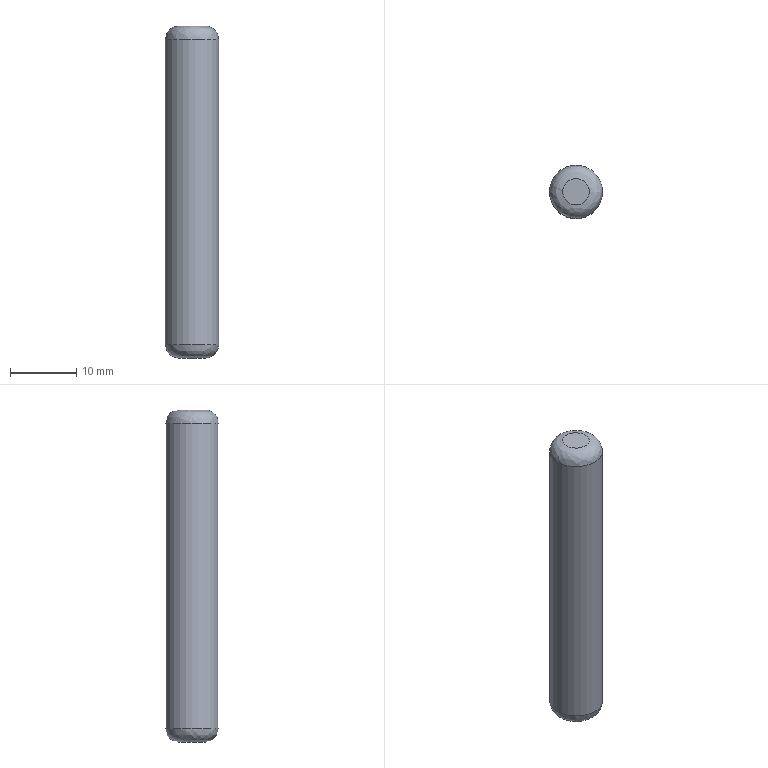Part | STEP file | 1 solid | 5 faces | box 8 x 8 x 50 mm | volume 2474 mm3 | plane 2 | spline 2 | cylinder 1 | commonest cylinder face diameters 8 x1
STEP:
#1=CARTESIAN_POINT('',(0.,0.,0.));
#2=DIRECTION('',(0.,0.,1.));
#3=DIRECTION('',(1.,0.,0.));
#4=AXIS2_PLACEMENT_3D('',#1,#2,#3);
#5=CARTESIAN_POINT('',(1296.247,499.955,58.619));
#6=VERTEX_POINT('',#5);
#7=CARTESIAN_POINT('',(1292.247,499.955,58.619));
#8=DIRECTION('',(0.,0.,-1.));
#9=DIRECTION('',(1.,0.,0.));
#10=AXIS2_PLACEMENT_3D('',#7,#8,#9);
#11=CIRCLE('',#10,4.);
#12=CARTESIAN_POINT('',(1292.247,499.955,10.619));
#13=DIRECTION('',(0.,0.,1.));
#14=DIRECTION('',(1.,0.,0.));
#15=AXIS2_PLACEMENT_3D('',#12,#13,#14);
#16=CYLINDRICAL_SURFACE('',#15,4.);
#17=CARTESIAN_POINT('',(6.283,48.));
#18=DIRECTION('',(-1.,0.));
#19=VECTOR('',#18,1.);
#20=LINE('',#17,#19);
#21=(GEOMETRIC_REPRESENTATION_CONTEXT(2)PARAMETRIC_REPRESENTATION_CONTEXT()REPRESENTATION_CONTEXT('',''));
#22=DEFINITIONAL_REPRESENTATION('',(#20),#21);
#23=PCURVE('',#16,#22);
#24=CARTESIAN_POINT('',(1288.247,499.955,58.619));
#25=CARTESIAN_POINT('',(1288.247,507.955,58.619));
#26=CARTESIAN_POINT('',(1296.247,507.955,58.619));
#27=CARTESIAN_POINT('',(1296.247,499.955,58.619));
#28=CARTESIAN_POINT('',(1296.247,491.955,58.619));
#29=CARTESIAN_POINT('',(1288.247,491.955,58.619));
#30=CARTESIAN_POINT('',(1288.247,499.955,58.619));
#31=CARTESIAN_POINT('',(1288.247,499.955,59.791));
#32=CARTESIAN_POINT('',(1288.247,507.955,59.791));
#33=CARTESIAN_POINT('',(1296.247,507.955,59.791));
#34=CARTESIAN_POINT('',(1296.247,499.955,59.791));
#35=CARTESIAN_POINT('',(1296.247,491.955,59.791));
#36=CARTESIAN_POINT('',(1288.247,491.955,59.791));
#37=CARTESIAN_POINT('',(1288.247,499.955,59.791));
#38=CARTESIAN_POINT('',(1289.076,499.955,60.619));
#39=CARTESIAN_POINT('',(1289.076,506.299,60.619));
#40=CARTESIAN_POINT('',(1295.419,506.299,60.619));
#41=CARTESIAN_POINT('',(1295.419,499.955,60.619));
#42=CARTESIAN_POINT('',(1295.419,493.612,60.619));
#43=CARTESIAN_POINT('',(1289.076,493.612,60.619));
#44=CARTESIAN_POINT('',(1289.076,499.955,60.619));
#45=CARTESIAN_POINT('',(1290.247,499.955,60.619));
#46=CARTESIAN_POINT('',(1290.247,503.955,60.619));
#47=CARTESIAN_POINT('',(1294.247,503.955,60.619));
#48=CARTESIAN_POINT('',(1294.247,499.955,60.619));
#49=CARTESIAN_POINT('',(1294.247,495.955,60.619));
#50=CARTESIAN_POINT('',(1290.247,495.955,60.619));
#51=CARTESIAN_POINT('',(1290.247,499.955,60.619));
#52=(BOUNDED_SURFACE()B_SPLINE_SURFACE(3,3,((#24,#25,#26,#27,#28,#29,#30),(#31,#32,#33,#34,#35,#36,#37),(#38,#39,#40,#41,#42,#43,#44),(#45,#46,#47,#48,#49,#50,#51)),.UNSPECIFIED.,.F.,.T.,.F.)B_SPLINE_SURFACE_WITH_KNOTS((4,4),(1,3,3,3,1),(0.,1.),(-0.5,0.,0.5,1.,1.5),.UNSPECIFIED.)GEOMETRIC_REPRESENTATION_ITEM()RATIONAL_B_SPLINE_SURFACE(((1.,0.3333,0.3333,1.,0.3333,0.3333,1.),(0.8047,0.2682,0.2682,0.8047,0.2682,0.2682,0.8047),(0.8047,0.2682,0.2682,0.8047,0.2682,0.2682,0.8047),(1.,0.3333,0.3333,1.,0.3333,0.3333,1.)))REPRESENTATION_ITEM('')SURFACE());
#53=CARTESIAN_POINT('',(0.,0.5));
#54=CARTESIAN_POINT('',(0.,0.5235));
#55=CARTESIAN_POINT('',(0.,0.5649));
#56=CARTESIAN_POINT('',(0.,0.6146));
#57=CARTESIAN_POINT('',(0.,0.6575));
#58=CARTESIAN_POINT('',(0.,0.696));
#59=CARTESIAN_POINT('',(0.,0.7322));
#60=CARTESIAN_POINT('',(0.,0.7678));
#61=CARTESIAN_POINT('',(0.,0.804));
#62=CARTESIAN_POINT('',(0.,0.8425));
#63=CARTESIAN_POINT('',(0.,0.8856));
#64=CARTESIAN_POINT('',(0.,0.9343));
#65=CARTESIAN_POINT('',(0.,1.));
#66=CARTESIAN_POINT('',(0.,1.066));
#67=CARTESIAN_POINT('',(0.,1.114));
#68=CARTESIAN_POINT('',(0.,1.158));
#69=CARTESIAN_POINT('',(0.,1.196));
#70=CARTESIAN_POINT('',(0.,1.232));
#71=CARTESIAN_POINT('',(0.,1.268));
#72=CARTESIAN_POINT('',(0.,1.304));
#73=CARTESIAN_POINT('',(0.,1.343));
#74=CARTESIAN_POINT('',(0.,1.385));
#75=CARTESIAN_POINT('',(0.,1.435));
#76=CARTESIAN_POINT('',(0.,1.476));
#77=CARTESIAN_POINT('',(0.,1.5));
#78=B_SPLINE_CURVE_WITH_KNOTS('',3,(#53,#54,#55,#56,#57,#58,#59,#60,#61,#62,#63,#64,#65,#66,#67,#68,#69,#70,#71,#72,#73,#74,#75,#76,#77),.UNSPECIFIED.,.F.,.F.,(4,1,1,1,1,1,1,1,1,1,1,1,1,1,1,1,1,1,1,1,1,1,4),(0.,0.2856,0.5712,0.8568,1.142,1.428,1.714,1.999,2.285,2.57,2.856,3.142,3.427,3.713,3.998,4.284,4.57,4.855,5.141,5.426,5.712,5.998,6.283),.QUASI_UNIFORM_KNOTS.);
#79=(GEOMETRIC_REPRESENTATION_CONTEXT(2)PARAMETRIC_REPRESENTATION_CONTEXT()REPRESENTATION_CONTEXT('',''));
#80=DEFINITIONAL_REPRESENTATION('',(#78),#79);
#81=PCURVE('',#52,#80);
#82=SURFACE_CURVE('',#11,(#23,#81),.PCURVE_S1.);
#83=EDGE_CURVE('',#6,#6,#82,.T.);
#84=ORIENTED_EDGE('',*,*,#83,.T.);
#85=CARTESIAN_POINT('',(1296.247,499.955,12.619));
#86=VERTEX_POINT('',#85);
#87=CARTESIAN_POINT('',(1296.247,499.955,12.619));
#88=CARTESIAN_POINT('',(1296.247,499.955,58.619));
#89=B_SPLINE_CURVE_WITH_KNOTS('',1,(#87,#88),.UNSPECIFIED.,.F.,.F.,(2,2),(2.,48.),.PIECEWISE_BEZIER_KNOTS.);
#90=CARTESIAN_POINT('',(0.,0.));
#91=DIRECTION('',(0.,1.));
#92=VECTOR('',#91,1.);
#93=LINE('',#90,#92);
#94=(GEOMETRIC_REPRESENTATION_CONTEXT(2)PARAMETRIC_REPRESENTATION_CONTEXT()REPRESENTATION_CONTEXT('',''));
#95=DEFINITIONAL_REPRESENTATION('',(#93),#94);
#96=PCURVE('',#16,#95);
#97=CARTESIAN_POINT('',(6.283,0.));
#98=DIRECTION('',(0.,1.));
#99=VECTOR('',#98,1.);
#100=LINE('',#97,#99);
#101=(GEOMETRIC_REPRESENTATION_CONTEXT(2)PARAMETRIC_REPRESENTATION_CONTEXT()REPRESENTATION_CONTEXT('',''));
#102=DEFINITIONAL_REPRESENTATION('',(#100),#101);
#103=PCURVE('',#16,#102);
#104=SEAM_CURVE('',#89,(#96,#103),.PCURVE_S1.);
#105=EDGE_CURVE('',#86,#6,#104,.T.);
#106=ORIENTED_EDGE('',*,*,#105,.F.);
#107=CARTESIAN_POINT('',(1292.247,499.955,12.619));
#108=DIRECTION('',(0.,0.,1.));
#109=DIRECTION('',(1.,0.,0.));
#110=AXIS2_PLACEMENT_3D('',#107,#108,#109);
#111=CIRCLE('',#110,4.);
#112=CARTESIAN_POINT('',(0.,2.));
#113=DIRECTION('',(1.,0.));
#114=VECTOR('',#113,1.);
#115=LINE('',#112,#114);
#116=(GEOMETRIC_REPRESENTATION_CONTEXT(2)PARAMETRIC_REPRESENTATION_CONTEXT()REPRESENTATION_CONTEXT('',''));
#117=DEFINITIONAL_REPRESENTATION('',(#115),#116);
#118=PCURVE('',#16,#117);
#119=CARTESIAN_POINT('',(1290.247,499.955,10.619));
#120=CARTESIAN_POINT('',(1290.247,503.955,10.619));
#121=CARTESIAN_POINT('',(1294.247,503.955,10.619));
#122=CARTESIAN_POINT('',(1294.247,499.955,10.619));
#123=CARTESIAN_POINT('',(1294.247,495.955,10.619));
#124=CARTESIAN_POINT('',(1290.247,495.955,10.619));
#125=CARTESIAN_POINT('',(1290.247,499.955,10.619));
#126=CARTESIAN_POINT('',(1289.076,499.955,10.619));
#127=CARTESIAN_POINT('',(1289.076,506.299,10.619));
#128=CARTESIAN_POINT('',(1295.419,506.299,10.619));
#129=CARTESIAN_POINT('',(1295.419,499.955,10.619));
#130=CARTESIAN_POINT('',(1295.419,493.612,10.619));
#131=CARTESIAN_POINT('',(1289.076,493.612,10.619));
#132=CARTESIAN_POINT('',(1289.076,499.955,10.619));
#133=CARTESIAN_POINT('',(1288.247,499.955,11.447));
#134=CARTESIAN_POINT('',(1288.247,507.955,11.447));
#135=CARTESIAN_POINT('',(1296.247,507.955,11.447));
#136=CARTESIAN_POINT('',(1296.247,499.955,11.447));
#137=CARTESIAN_POINT('',(1296.247,491.955,11.447));
#138=CARTESIAN_POINT('',(1288.247,491.955,11.447));
#139=CARTESIAN_POINT('',(1288.247,499.955,11.447));
#140=CARTESIAN_POINT('',(1288.247,499.955,12.619));
#141=CARTESIAN_POINT('',(1288.247,507.955,12.619));
#142=CARTESIAN_POINT('',(1296.247,507.955,12.619));
#143=CARTESIAN_POINT('',(1296.247,499.955,12.619));
#144=CARTESIAN_POINT('',(1296.247,491.955,12.619));
#145=CARTESIAN_POINT('',(1288.247,491.955,12.619));
#146=CARTESIAN_POINT('',(1288.247,499.955,12.619));
#147=(BOUNDED_SURFACE()B_SPLINE_SURFACE(3,3,((#119,#120,#121,#122,#123,#124,#125),(#126,#127,#128,#129,#130,#131,#132),(#133,#134,#135,#136,#137,#138,#139),(#140,#141,#142,#143,#144,#145,#146)),.UNSPECIFIED.,.F.,.T.,.F.)B_SPLINE_SURFACE_WITH_KNOTS((4,4),(1,3,3,3,1),(0.,1.),(-0.5,0.,0.5,1.,1.5),.UNSPECIFIED.)GEOMETRIC_REPRESENTATION_ITEM()RATIONAL_B_SPLINE_SURFACE(((1.,0.3333,0.3333,1.,0.3333,0.3333,1.),(0.8047,0.2682,0.2682,0.8047,0.2682,0.2682,0.8047),(0.8047,0.2682,0.2682,0.8047,0.2682,0.2682,0.8047),(1.,0.3333,0.3333,1.,0.3333,0.3333,1.)))REPRESENTATION_ITEM('')SURFACE());
#148=CARTESIAN_POINT('',(1.,1.5));
#149=CARTESIAN_POINT('',(1.,1.476));
#150=CARTESIAN_POINT('',(1.,1.435));
#151=CARTESIAN_POINT('',(1.,1.385));
#152=CARTESIAN_POINT('',(1.,1.343));
#153=CARTESIAN_POINT('',(1.,1.304));
#154=CARTESIAN_POINT('',(1.,1.268));
#155=CARTESIAN_POINT('',(1.,1.232));
#156=CARTESIAN_POINT('',(1.,1.196));
#157=CARTESIAN_POINT('',(1.,1.158));
#158=CARTESIAN_POINT('',(1.,1.114));
#159=CARTESIAN_POINT('',(1.,1.066));
#160=CARTESIAN_POINT('',(1.,1.));
#161=CARTESIAN_POINT('',(1.,0.9343));
#162=CARTESIAN_POINT('',(1.,0.8856));
#163=CARTESIAN_POINT('',(1.,0.8425));
#164=CARTESIAN_POINT('',(1.,0.804));
#165=CARTESIAN_POINT('',(1.,0.7678));
#166=CARTESIAN_POINT('',(1.,0.7322));
#167=CARTESIAN_POINT('',(1.,0.696));
#168=CARTESIAN_POINT('',(1.,0.6575));
#169=CARTESIAN_POINT('',(1.,0.6146));
#170=CARTESIAN_POINT('',(1.,0.5649));
#171=CARTESIAN_POINT('',(1.,0.5235));
#172=CARTESIAN_POINT('',(1.,0.5));
#173=B_SPLINE_CURVE_WITH_KNOTS('',3,(#148,#149,#150,#151,#152,#153,#154,#155,#156,#157,#158,#159,#160,#161,#162,#163,#164,#165,#166,#167,#168,#169,#170,#171,#172),.UNSPECIFIED.,.F.,.F.,(4,1,1,1,1,1,1,1,1,1,1,1,1,1,1,1,1,1,1,1,1,1,4),(0.,0.2856,0.5712,0.8568,1.142,1.428,1.714,1.999,2.285,2.57,2.856,3.142,3.427,3.713,3.998,4.284,4.57,4.855,5.141,5.426,5.712,5.998,6.283),.QUASI_UNIFORM_KNOTS.);
#174=(GEOMETRIC_REPRESENTATION_CONTEXT(2)PARAMETRIC_REPRESENTATION_CONTEXT()REPRESENTATION_CONTEXT('',''));
#175=DEFINITIONAL_REPRESENTATION('',(#173),#174);
#176=PCURVE('',#147,#175);
#177=SURFACE_CURVE('',#111,(#118,#176),.PCURVE_S1.);
#178=EDGE_CURVE('',#86,#86,#177,.T.);
#179=ORIENTED_EDGE('',*,*,#178,.T.);
#180=ORIENTED_EDGE('',*,*,#105,.T.);
#181=EDGE_LOOP('',(#84,#106,#179,#180));
#182=FACE_BOUND('',#181,.T.);
#183=ADVANCED_FACE('',(#182),#16,.T.);
#184=CARTESIAN_POINT('',(1294.247,499.955,10.619));
#185=VERTEX_POINT('',#184);
#186=CARTESIAN_POINT('',(1292.247,499.955,10.619));
#187=DIRECTION('',(0.,0.,-1.));
#188=DIRECTION('',(1.,0.,0.));
#189=AXIS2_PLACEMENT_3D('',#186,#187,#188);
#190=CIRCLE('',#189,2.);
#191=CARTESIAN_POINT('',(1292.247,499.955,10.619));
#192=DIRECTION('',(0.,0.,-1.));
#193=DIRECTION('',(-1.,0.,0.));
#194=AXIS2_PLACEMENT_3D('',#191,#192,#193);
#195=PLANE('',#194);
#196=CARTESIAN_POINT('',(0.,0.));
#197=DIRECTION('',(-1.,0.));
#198=AXIS2_PLACEMENT_2D('',#196,#197);
#199=CIRCLE('',#198,2.);
#200=(GEOMETRIC_REPRESENTATION_CONTEXT(2)PARAMETRIC_REPRESENTATION_CONTEXT()REPRESENTATION_CONTEXT('',''));
#201=DEFINITIONAL_REPRESENTATION('',(#199),#200);
#202=PCURVE('',#195,#201);
#203=CARTESIAN_POINT('',(0.,0.5));
#204=CARTESIAN_POINT('',(0.,0.5235));
#205=CARTESIAN_POINT('',(0.,0.5649));
#206=CARTESIAN_POINT('',(0.,0.6146));
#207=CARTESIAN_POINT('',(0.,0.6575));
#208=CARTESIAN_POINT('',(0.,0.696));
#209=CARTESIAN_POINT('',(0.,0.7322));
#210=CARTESIAN_POINT('',(0.,0.7678));
#211=CARTESIAN_POINT('',(0.,0.804));
#212=CARTESIAN_POINT('',(0.,0.8425));
#213=CARTESIAN_POINT('',(0.,0.8856));
#214=CARTESIAN_POINT('',(0.,0.9343));
#215=CARTESIAN_POINT('',(0.,1.));
#216=CARTESIAN_POINT('',(0.,1.066));
#217=CARTESIAN_POINT('',(0.,1.114));
#218=CARTESIAN_POINT('',(0.,1.158));
#219=CARTESIAN_POINT('',(0.,1.196));
#220=CARTESIAN_POINT('',(0.,1.232));
#221=CARTESIAN_POINT('',(0.,1.268));
#222=CARTESIAN_POINT('',(0.,1.304));
#223=CARTESIAN_POINT('',(0.,1.343));
#224=CARTESIAN_POINT('',(0.,1.385));
#225=CARTESIAN_POINT('',(0.,1.435));
#226=CARTESIAN_POINT('',(0.,1.476));
#227=CARTESIAN_POINT('',(0.,1.5));
#228=B_SPLINE_CURVE_WITH_KNOTS('',3,(#203,#204,#205,#206,#207,#208,#209,#210,#211,#212,#213,#214,#215,#216,#217,#218,#219,#220,#221,#222,#223,#224,#225,#226,#227),.UNSPECIFIED.,.F.,.F.,(4,1,1,1,1,1,1,1,1,1,1,1,1,1,1,1,1,1,1,1,1,1,4),(0.,0.2856,0.5712,0.8568,1.142,1.428,1.714,1.999,2.285,2.57,2.856,3.142,3.427,3.713,3.998,4.284,4.57,4.855,5.141,5.426,5.712,5.998,6.283),.QUASI_UNIFORM_KNOTS.);
#229=(GEOMETRIC_REPRESENTATION_CONTEXT(2)PARAMETRIC_REPRESENTATION_CONTEXT()REPRESENTATION_CONTEXT('',''));
#230=DEFINITIONAL_REPRESENTATION('',(#228),#229);
#231=PCURVE('',#147,#230);
#232=SURFACE_CURVE('',#190,(#202,#231),.PCURVE_S1.);
#233=EDGE_CURVE('',#185,#185,#232,.T.);
#234=ORIENTED_EDGE('',*,*,#233,.T.);
#235=EDGE_LOOP('',(#234));
#236=FACE_BOUND('',#235,.T.);
#237=ADVANCED_FACE('',(#236),#195,.T.);
#238=CARTESIAN_POINT('',(1294.247,499.955,60.619));
#239=VERTEX_POINT('',#238);
#240=CARTESIAN_POINT('',(1292.247,499.955,60.619));
#241=DIRECTION('',(0.,0.,1.));
#242=DIRECTION('',(1.,0.,0.));
#243=AXIS2_PLACEMENT_3D('',#240,#241,#242);
#244=CIRCLE('',#243,2.);
#245=CARTESIAN_POINT('',(1292.247,499.955,60.619));
#246=DIRECTION('',(0.,0.,-1.));
#247=DIRECTION('',(-1.,0.,0.));
#248=AXIS2_PLACEMENT_3D('',#245,#246,#247);
#249=PLANE('',#248);
#250=CARTESIAN_POINT('',(-2.,0.));
#251=CARTESIAN_POINT('',(-2.,3.464));
#252=CARTESIAN_POINT('',(1.,1.732));
#253=CARTESIAN_POINT('',(4.,0.));
#254=CARTESIAN_POINT('',(1.,-1.732));
#255=CARTESIAN_POINT('',(-2.,-3.464));
#256=CARTESIAN_POINT('',(-2.,0.));
#257=(BOUNDED_CURVE()B_SPLINE_CURVE(2,(#250,#251,#252,#253,#254,#255,#256),.UNSPECIFIED.,.T.,.F.)B_SPLINE_CURVE_WITH_KNOTS((1,2,2,2,2,1),(-2.094,0.,2.094,4.189,6.283,8.378),.UNSPECIFIED.)CURVE()GEOMETRIC_REPRESENTATION_ITEM()RATIONAL_B_SPLINE_CURVE((1.,0.5,1.,0.5,1.,0.5,1.))REPRESENTATION_ITEM(''));
#258=(GEOMETRIC_REPRESENTATION_CONTEXT(2)PARAMETRIC_REPRESENTATION_CONTEXT()REPRESENTATION_CONTEXT('',''));
#259=DEFINITIONAL_REPRESENTATION('',(#257),#258);
#260=PCURVE('',#249,#259);
#261=CARTESIAN_POINT('',(1.,1.5));
#262=CARTESIAN_POINT('',(1.,1.476));
#263=CARTESIAN_POINT('',(1.,1.435));
#264=CARTESIAN_POINT('',(1.,1.385));
#265=CARTESIAN_POINT('',(1.,1.343));
#266=CARTESIAN_POINT('',(1.,1.304));
#267=CARTESIAN_POINT('',(1.,1.268));
#268=CARTESIAN_POINT('',(1.,1.232));
#269=CARTESIAN_POINT('',(1.,1.196));
#270=CARTESIAN_POINT('',(1.,1.158));
#271=CARTESIAN_POINT('',(1.,1.114));
#272=CARTESIAN_POINT('',(1.,1.066));
#273=CARTESIAN_POINT('',(1.,1.));
#274=CARTESIAN_POINT('',(1.,0.9343));
#275=CARTESIAN_POINT('',(1.,0.8856));
#276=CARTESIAN_POINT('',(1.,0.8425));
#277=CARTESIAN_POINT('',(1.,0.804));
#278=CARTESIAN_POINT('',(1.,0.7678));
#279=CARTESIAN_POINT('',(1.,0.7322));
#280=CARTESIAN_POINT('',(1.,0.696));
#281=CARTESIAN_POINT('',(1.,0.6575));
#282=CARTESIAN_POINT('',(1.,0.6146));
#283=CARTESIAN_POINT('',(1.,0.5649));
#284=CARTESIAN_POINT('',(1.,0.5235));
#285=CARTESIAN_POINT('',(1.,0.5));
#286=B_SPLINE_CURVE_WITH_KNOTS('',3,(#261,#262,#263,#264,#265,#266,#267,#268,#269,#270,#271,#272,#273,#274,#275,#276,#277,#278,#279,#280,#281,#282,#283,#284,#285),.UNSPECIFIED.,.F.,.F.,(4,1,1,1,1,1,1,1,1,1,1,1,1,1,1,1,1,1,1,1,1,1,4),(0.,0.2856,0.5712,0.8568,1.142,1.428,1.714,1.999,2.285,2.57,2.856,3.142,3.427,3.713,3.998,4.284,4.57,4.855,5.141,5.426,5.712,5.998,6.283),.QUASI_UNIFORM_KNOTS.);
#287=(GEOMETRIC_REPRESENTATION_CONTEXT(2)PARAMETRIC_REPRESENTATION_CONTEXT()REPRESENTATION_CONTEXT('',''));
#288=DEFINITIONAL_REPRESENTATION('',(#286),#287);
#289=PCURVE('',#52,#288);
#290=SURFACE_CURVE('',#244,(#260,#289),.PCURVE_S1.);
#291=EDGE_CURVE('',#239,#239,#290,.T.);
#292=ORIENTED_EDGE('',*,*,#291,.T.);
#293=EDGE_LOOP('',(#292));
#294=FACE_BOUND('',#293,.T.);
#295=ADVANCED_FACE('',(#294),#249,.F.);
#296=ORIENTED_EDGE('',*,*,#291,.F.);
#297=CARTESIAN_POINT('',(1296.247,499.955,58.619));
#298=CARTESIAN_POINT('',(1296.247,499.955,59.791));
#299=CARTESIAN_POINT('',(1295.419,499.955,60.619));
#300=CARTESIAN_POINT('',(1294.247,499.955,60.619));
#301=(BOUNDED_CURVE()B_SPLINE_CURVE(3,(#297,#298,#299,#300),.UNSPECIFIED.,.F.,.F.)B_SPLINE_CURVE_WITH_KNOTS((4,4),(0.,1.),.PIECEWISE_BEZIER_KNOTS.)CURVE()GEOMETRIC_REPRESENTATION_ITEM()RATIONAL_B_SPLINE_CURVE((1.,0.8047,0.8047,1.))REPRESENTATION_ITEM(''));
#302=CARTESIAN_POINT('',(0.,1.5));
#303=DIRECTION('',(1.,0.));
#304=VECTOR('',#303,1.);
#305=LINE('',#302,#304);
#306=(GEOMETRIC_REPRESENTATION_CONTEXT(2)PARAMETRIC_REPRESENTATION_CONTEXT()REPRESENTATION_CONTEXT('',''));
#307=DEFINITIONAL_REPRESENTATION('',(#305),#306);
#308=PCURVE('',#52,#307);
#309=CARTESIAN_POINT('',(0.,0.5));
#310=DIRECTION('',(1.,0.));
#311=VECTOR('',#310,1.);
#312=LINE('',#309,#311);
#313=(GEOMETRIC_REPRESENTATION_CONTEXT(2)PARAMETRIC_REPRESENTATION_CONTEXT()REPRESENTATION_CONTEXT('',''));
#314=DEFINITIONAL_REPRESENTATION('',(#312),#313);
#315=PCURVE('',#52,#314);
#316=SEAM_CURVE('',#301,(#308,#315),.PCURVE_S1.);
#317=EDGE_CURVE('',#6,#239,#316,.T.);
#318=ORIENTED_EDGE('',*,*,#317,.F.);
#319=ORIENTED_EDGE('',*,*,#83,.F.);
#320=ORIENTED_EDGE('',*,*,#317,.T.);
#321=EDGE_LOOP('',(#296,#318,#319,#320));
#322=FACE_BOUND('',#321,.T.);
#323=ADVANCED_FACE('',(#322),#52,.T.);
#324=ORIENTED_EDGE('',*,*,#178,.F.);
#325=CARTESIAN_POINT('',(1294.247,499.955,10.619));
#326=CARTESIAN_POINT('',(1295.419,499.955,10.619));
#327=CARTESIAN_POINT('',(1296.247,499.955,11.447));
#328=CARTESIAN_POINT('',(1296.247,499.955,12.619));
#329=(BOUNDED_CURVE()B_SPLINE_CURVE(3,(#325,#326,#327,#328),.UNSPECIFIED.,.F.,.F.)B_SPLINE_CURVE_WITH_KNOTS((4,4),(0.,1.),.PIECEWISE_BEZIER_KNOTS.)CURVE()GEOMETRIC_REPRESENTATION_ITEM()RATIONAL_B_SPLINE_CURVE((1.,0.8047,0.8047,1.))REPRESENTATION_ITEM(''));
#330=CARTESIAN_POINT('',(0.,1.5));
#331=DIRECTION('',(1.,0.));
#332=VECTOR('',#331,1.);
#333=LINE('',#330,#332);
#334=(GEOMETRIC_REPRESENTATION_CONTEXT(2)PARAMETRIC_REPRESENTATION_CONTEXT()REPRESENTATION_CONTEXT('',''));
#335=DEFINITIONAL_REPRESENTATION('',(#333),#334);
#336=PCURVE('',#147,#335);
#337=CARTESIAN_POINT('',(0.,0.5));
#338=DIRECTION('',(1.,0.));
#339=VECTOR('',#338,1.);
#340=LINE('',#337,#339);
#341=(GEOMETRIC_REPRESENTATION_CONTEXT(2)PARAMETRIC_REPRESENTATION_CONTEXT()REPRESENTATION_CONTEXT('',''));
#342=DEFINITIONAL_REPRESENTATION('',(#340),#341);
#343=PCURVE('',#147,#342);
#344=SEAM_CURVE('',#329,(#336,#343),.PCURVE_S1.);
#345=EDGE_CURVE('',#185,#86,#344,.T.);
#346=ORIENTED_EDGE('',*,*,#345,.F.);
#347=ORIENTED_EDGE('',*,*,#233,.F.);
#348=ORIENTED_EDGE('',*,*,#345,.T.);
#349=EDGE_LOOP('',(#324,#346,#347,#348));
#350=FACE_BOUND('',#349,.T.);
#351=ADVANCED_FACE('',(#350),#147,.T.);
#352=CLOSED_SHELL('',(#183,#237,#295,#323,#351));
#353=MANIFOLD_SOLID_BREP('',#352);
#354=(LENGTH_UNIT()NAMED_UNIT(*)SI_UNIT(.MILLI.,.METRE.));
#355=UNCERTAINTY_MEASURE_WITH_UNIT(LENGTH_MEASURE(0.00001),#354,'','');
#356=(NAMED_UNIT(*)PLANE_ANGLE_UNIT()SI_UNIT($,.RADIAN.));
#357=(NAMED_UNIT(*)SI_UNIT($,.STERADIAN.)SOLID_ANGLE_UNIT());
#358=(GEOMETRIC_REPRESENTATION_CONTEXT(3)GLOBAL_UNCERTAINTY_ASSIGNED_CONTEXT((#355))GLOBAL_UNIT_ASSIGNED_CONTEXT((#354,#356,#357))REPRESENTATION_CONTEXT('',''));
#359=ADVANCED_BREP_SHAPE_REPRESENTATION('',(#4,#353),#358);